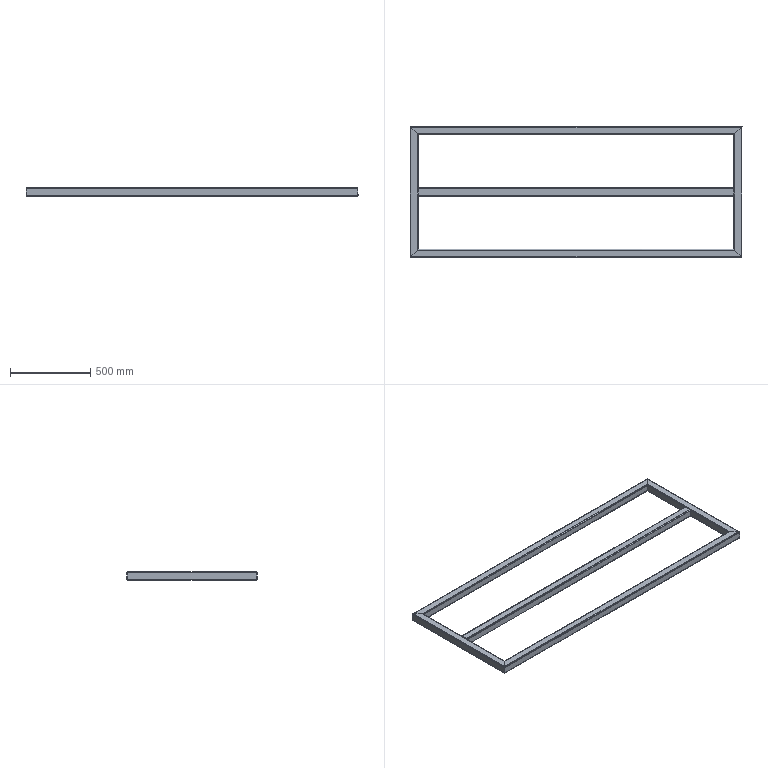Part | SolidWorks | 5 solids | 90 faces | box 2070 x 815 x 50 mm | volume 4077805 mm3 | plane 50 | cylinder 40 | commonest cylinder face diameters 6 x20 12 x20